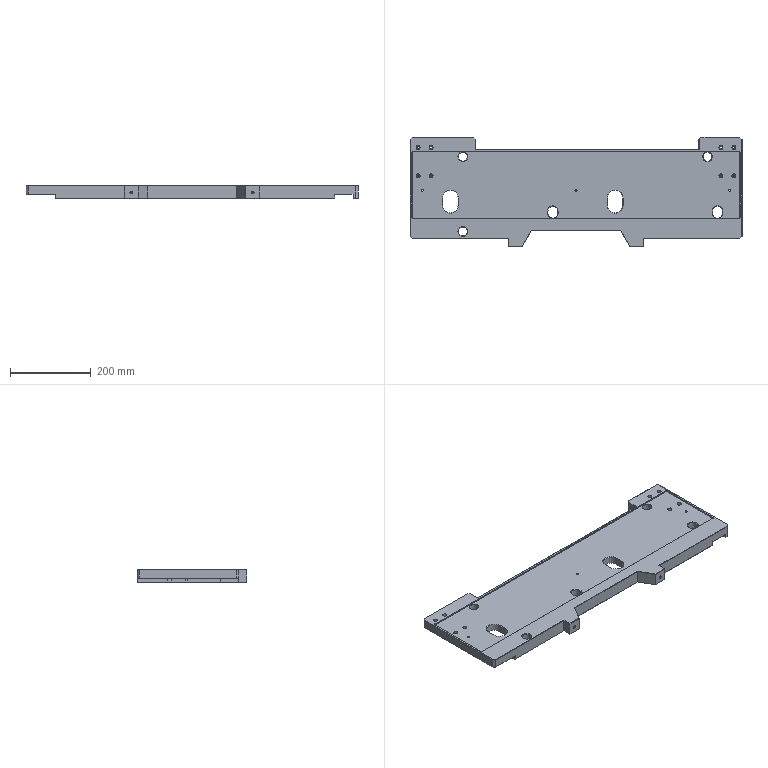Part | SolidWorks | features ICE 22, Chamfer 16, 3DProfileFeature 11, HoleWzd 11, Fillet 3, LPattern 2, Extrusion 1 | 1 solid | 361 faces | box 820.75 x 270 x 32.5 mm | volume 4272161 mm3 | plane 165 | cylinder 116 | cone 80 | commonest cylinder face diameters 5 x26 10 x23 3.3 x16 5.5 x16 4.2 x12 22 x6